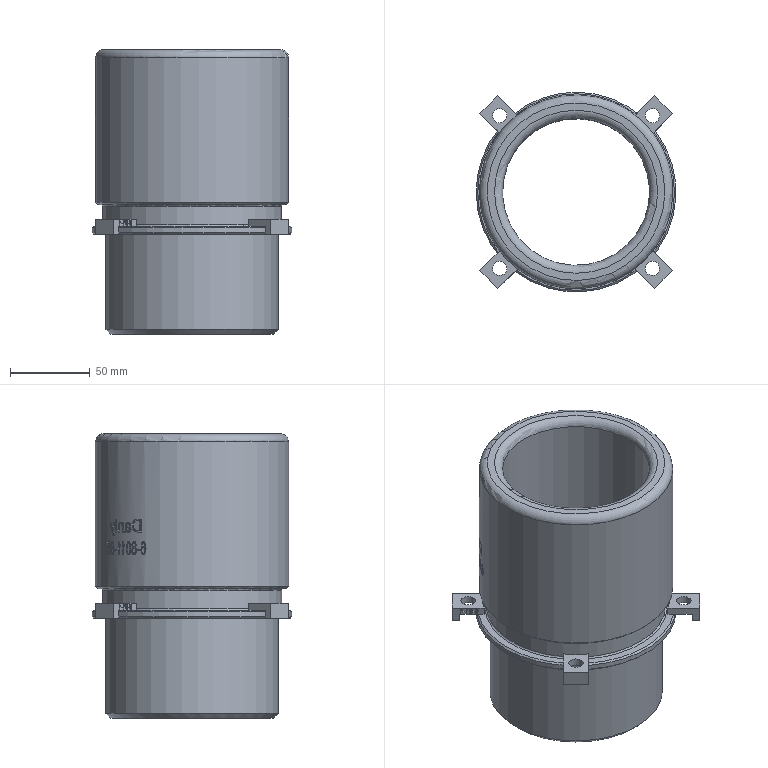Part | STEP file | lll_id4482_x_t | 1 solid | 351 faces | box 125 x 125 x 178 mm | volume 698493 mm3 | plane 204 | other 121 | cylinder 17 | torus 5 | cone 4 | commonest cylinder face diameters 121 x9 9 x4 92 x1 108 x1 112 x1 125 x1